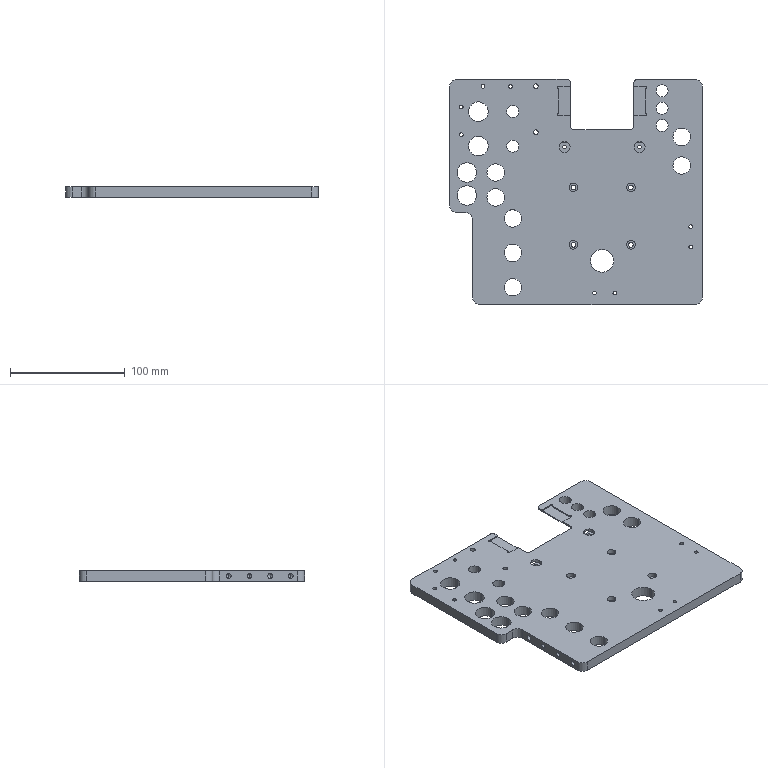NC program | NX | posted with a generic post | part box 220 x 196 x 9 mm
Lines 131 to 1017 of 7489:
(ZLEVEL_PROFILE , TOOL : D10)
N236 T15 M6
N238 G54
N240 G17 G0 G90 X56.431 Y-103.1 S9500 M3
N242 G43 Z30. H15
N244 Z1.5
N246 G94 G1 X10. Z-0.933 F1000.
N248 X-84. F3200.
N250 G2 X-95.1 Y-92. R11.1
N252 G1 Y-24.
N254 G3 X-96. Y-23.1 R0.9
N256 G1 X-104.
N258 G2 X-115.1 Y-12. R11.1
N260 G1 Y92.
N262 G2 X-104. Y103.1 R11.1
N264 G1 X-7.8
N266 G2 X0.3 Y95. R8.1
N268 G1 Y92.
N270 G2 X0.275 Y91.491 R5.1
N272 G1 Y66.909
N274 G2 X0.3 Y66.4 R5.1
N276 G1 Y59.5
N278 X45.15
N280 Y66.4
N282 G2 X45.175 Y66.909 R5.1
N284 G1 Y91.491
N286 G2 X45.15 Y92. R5.1
N288 G1 Y95.
N290 G2 X53.25 Y103.1 R8.1
N292 G1 X104.
N294 G2 X115.1 Y92. R11.1
N296 G1 Y-92.
N298 G2 X104. Y-103.1 R11.1
N300 G1 X10.
N302 X-43.471 Z-1.867
N304 X-84.
N306 G2 X-95.1 Y-92. R11.1
N308 G1 Y-24.
N310 G3 X-96. Y-23.1 R0.9
N312 G1 X-104.
N314 G2 X-115.1 Y-12. R11.1
N316 G1 Y92.
N318 G2 X-104. Y103.1 R11.1
N320 G1 X-7.8
N322 G2 X0.3 Y95. R8.1
N324 G1 Y59.5
N326 X45.15
N328 Y95.
N330 G2 X53.25 Y103.1 R8.1
N332 G1 X104.
N334 G2 X115.1 Y92. R11.1
N336 G1 Y-92.
N338 G2 X104. Y-103.1 R11.1
N340 G1 X10.
N342 X-43.471 Z-2.8
N344 X-84.
N346 G2 X-95.1 Y-92. R11.1
N348 G1 Y-24.
N350 G3 X-96. Y-23.1 R0.9
N352 G1 X-104.
N354 G2 X-115.1 Y-12. R11.1
N356 G1 Y92.
N358 G2 X-104. Y103.1 R11.1
N360 G1 X-7.8
N362 G2 X0.3 Y95. R8.1
N364 G1 Y59.5
N366 X45.15
N368 Y95.
N370 G2 X53.25 Y103.1 R8.1
N372 G1 X104.
N374 G2 X115.1 Y92. R11.1
N376 G1 Y-92.
N378 G2 X104. Y-103.1 R11.1
N380 G1 X10.
N382 X-43.471 Z-3.733
N384 X-84.
N386 G2 X-95.1 Y-92. R11.1
N388 G1 Y-24.
N390 G3 X-96. Y-23.1 R0.9
N392 G1 X-104.
N394 G2 X-115.1 Y-12. R11.1
N396 G1 Y92.
N398 G2 X-104. Y103.1 R11.1
N400 G1 X-7.8
N402 G2 X0.3 Y95. R8.1
N404 G1 Y59.5
N406 X45.15
N408 Y95.
N410 G2 X53.25 Y103.1 R8.1
N412 G1 X104.
N414 G2 X115.1 Y92. R11.1
N416 G1 Y-92.
N418 G2 X104. Y-103.1 R11.1
N420 G1 X10.
N422 X-43.471 Z-4.667
N424 X-84.
N426 G2 X-95.1 Y-92. R11.1
N428 G1 Y-24.
N430 G3 X-96. Y-23.1 R0.9
N432 G1 X-104.
N434 G2 X-115.1 Y-12. R11.1
N436 G1 Y92.
N438 G2 X-104. Y103.1 R11.1
N440 G1 X-7.8
N442 G2 X0.3 Y95. R8.1
N444 G1 Y59.5
N446 X45.15
N448 Y95.
N450 G2 X53.25 Y103.1 R8.1
N452 G1 X104.
N454 G2 X115.1 Y92. R11.1
N456 G1 Y-92.
N458 G2 X104. Y-103.1 R11.1
N460 G1 X10.
N462 X-43.471 Z-5.6
N464 X-84.
N466 G2 X-95.1 Y-92. R11.1
N468 G1 Y-24.
N470 G3 X-96. Y-23.1 R0.9
N472 G1 X-104.
N474 G2 X-115.1 Y-12. R11.1
N476 G1 Y92.
N478 G2 X-104. Y103.1 R11.1
N480 G1 X-7.8
N482 G2 X0.3 Y95. R8.1
N484 G1 Y59.5
N486 X45.15
N488 Y95.
N490 G2 X53.25 Y103.1 R8.1
N492 G1 X104.
N494 G2 X115.1 Y92. R11.1
N496 G1 Y-92.
N498 G2 X104. Y-103.1 R11.1
N500 G1 X10.
N502 X-43.471 Z-6.533
N504 X-84.
N506 G2 X-95.1 Y-92. R11.1
N508 G1 Y-24.
N510 G3 X-96. Y-23.1 R0.9
N512 G1 X-104.
N514 G2 X-115.1 Y-12. R11.1
N516 G1 Y92.
N518 G2 X-104. Y103.1 R11.1
N520 G1 X-7.8
N522 G2 X0.3 Y95. R8.1
N524 G1 Y59.5
N526 X45.15
N528 Y95.
N530 G2 X53.25 Y103.1 R8.1
N532 G1 X104.
N534 G2 X115.1 Y92. R11.1
N536 G1 Y-92.
N538 G2 X104. Y-103.1 R11.1
N540 G1 X10.
N542 X-43.471 Z-7.467
N544 X-84.
N546 G2 X-95.1 Y-92. R11.1
N548 G1 Y-24.
N550 G3 X-96. Y-23.1 R0.9
N552 G1 X-104.
N554 G2 X-115.1 Y-12. R11.1
N556 G1 Y92.
N558 G2 X-104. Y103.1 R11.1
N560 G1 X-7.8
N562 G2 X0.3 Y95. R8.1
N564 G1 Y59.5
N566 X45.15
N568 Y95.
N570 G2 X53.25 Y103.1 R8.1
N572 G1 X104.
N574 G2 X115.1 Y92. R11.1
N576 G1 Y-92.
N578 G2 X104. Y-103.1 R11.1
N580 G1 X10.
N582 X-43.471 Z-8.4
N584 X-84.
N586 G2 X-95.1 Y-92. R11.1
N588 G1 Y-24.
N590 G3 X-96. Y-23.1 R0.9
N592 G1 X-104.
N594 G2 X-115.1 Y-12. R11.1
N596 G1 Y92.
N598 G2 X-104. Y103.1 R11.1
N600 G1 X-7.8
N602 G2 X0.3 Y95. R8.1
N604 G1 Y59.5
N606 X45.15
N608 Y95.
N610 G2 X53.25 Y103.1 R8.1
N612 G1 X104.
N614 G2 X115.1 Y92. R11.1
N616 G1 Y-92.
N618 G2 X104. Y-103.1 R11.1
N620 G1 X-43.471
N622 Z-6.9
N624 G0 Z30.
(ZLEVEL_PROFILE_COPY , TOOL : D10)
N626 X-85.581 Y73.328
N628 Z1.5
N630 G1 X-86.277 Y73.183 Z1.463 F1000.
N632 X-87.297 Y72.547 Z1.4
N634 X-88.035 Y71.598 Z1.337
N636 X-88.4 Y70.453 Z1.274
N638 Y69.995 Z1.25
N640 X-88.399 Y69.543 Z1.226
N642 X-88.219 Y68.816 Z1.187
N644 X-87.797 Y68.015 Z1.139
N646 X-87.016 Y67.225 Z1.081
N648 X-86.024 Y66.727 Z1.023
N650 X-84.925 Y66.571 Z0.965
N652 X-83.833 Y66.774 Z0.907
N654 X-82.864 Y67.316 Z0.848
N656 X-82.236 Y67.968 Z0.801
N658 X-81.82 Y68.716 Z0.756
N660 X-81.601 Y69.543 Z0.711
N662 X-81.599 Y70.448 Z0.664
N664 X-81.861 Y71.383 Z0.613
N666 X-82.375 Y72.207 Z0.562
N668 X-83.098 Y72.855 Z0.511
N670 X-83.911 Y73.253 Z0.464
N672 X-85.101 Y73.429 Z0.401
N674 X-86.277 Y73.183 Z0.338
N676 X-87.297 Y72.547 Z0.275
N678 X-88.035 Y71.598 Z0.212
N680 X-88.4 Y70.453 Z0.149
N682 Y69.995 Z0.125
N684 X-88.399 Y69.543 Z0.101
N686 X-88.219 Y68.816 Z0.062
N688 X-87.797 Y68.015 Z0.014
N690 X-87.016 Y67.225 Z-0.044
N692 X-86.024 Y66.727 Z-0.102
N694 X-84.925 Y66.571 Z-0.16
N696 X-83.833 Y66.774 Z-0.218
N698 X-82.864 Y67.316 Z-0.277
N700 X-82.236 Y67.968 Z-0.324
N702 X-81.82 Y68.716 Z-0.369
N704 X-81.601 Y69.543 Z-0.414
N706 X-81.599 Y70.448 Z-0.461
N708 X-81.861 Y71.383 Z-0.512
N710 X-82.375 Y72.207 Z-0.563
N712 X-83.098 Y72.855 Z-0.614
N714 X-83.911 Y73.253 Z-0.661
N716 X-85.101 Y73.429 Z-0.724
N718 X-86.277 Y73.183 Z-0.787
N720 X-87.297 Y72.547 Z-0.85
N722 X-88.035 Y71.598 Z-0.913
N724 X-88.4 Y70.453 Z-0.976
N726 Y70. Z-1.
N728 Y69.995 F2000.
N730 G3 X-84.995 Y66.6 R3.4
N732 X-88.4 Y70. R-3.4
N734 G1 X-88.383 Y69.661 Z-1.021
N736 X-88.348 Y69.41 Z-1.037
N738 X-88.315 Y69.243 Z-1.048
N740 X-88.23 Y68.939 Z-1.067
N742 X-88.142 Y68.701 Z-1.083
N744 X-88.063 Y68.525 Z-1.095
N746 X-87.915 Y68.25 Z-1.115
N748 X-87.776 Y68.037 Z-1.131
N750 X-87.658 Y67.88 Z-1.143
N752 X-87.453 Y67.645 Z-1.162
N754 X-87.27 Y67.469 Z-1.178
N756 X-87.12 Y67.342 Z-1.19
N758 X-86.867 Y67.159 Z-1.21
N760 X-86.65 Y67.027 Z-1.226
N762 X-86.475 Y66.937 Z-1.238
N764 X-86.188 Y66.814 Z-1.258
N766 X-85.947 Y66.735 Z-1.273
N768 X-85.757 Y66.685 Z-1.286
N770 X-85.449 Y66.63 Z-1.305
N772 X-85.197 Y66.606 Z-1.321
N774 X-85. Y66.6 Z-1.333
N776 X-84.688 Y66.614 Z-1.353
N778 X-84.436 Y66.647 Z-1.369
N780 X-84.243 Y66.685 Z-1.381
N782 X-83.943 Y66.769 Z-1.4
N784 X-83.704 Y66.857 Z-1.416
N786 X-83.525 Y66.937 Z-1.429
N788 X-83.25 Y67.085 Z-1.448
N790 X-83.037 Y67.224 Z-1.464
N792 X-82.88 Y67.342 Z-1.476
N794 X-82.645 Y67.547 Z-1.496
N796 X-82.469 Y67.73 Z-1.512
N798 X-82.342 Y67.88 Z-1.524
N800 X-82.159 Y68.133 Z-1.543
N802 X-82.027 Y68.35 Z-1.559
N804 X-81.937 Y68.525 Z-1.571
N806 X-81.814 Y68.812 Z-1.591
N808 X-81.735 Y69.053 Z-1.607
N810 X-81.685 Y69.243 Z-1.619
N812 X-81.63 Y69.551 Z-1.638
N814 X-81.606 Y69.803 Z-1.654
N816 X-81.6 Y70. Z-1.667
N818 X-81.614 Y70.312 Z-1.686
N820 X-81.647 Y70.564 Z-1.702
N822 X-81.685 Y70.757 Z-1.714
N824 X-81.769 Y71.057 Z-1.734
N826 X-81.857 Y71.296 Z-1.75
N828 X-81.937 Y71.475 Z-1.762
N830 X-82.085 Y71.75 Z-1.781
N832 X-82.224 Y71.963 Z-1.797
N834 X-82.342 Y72.12 Z-1.81
N836 X-82.547 Y72.355 Z-1.829
N838 X-82.73 Y72.531 Z-1.845
N840 X-82.88 Y72.658 Z-1.857
N842 X-83.133 Y72.841 Z-1.877
N844 X-83.35 Y72.973 Z-1.892
N846 X-83.525 Y73.063 Z-1.905
N848 X-83.812 Y73.186 Z-1.924
N850 X-84.053 Y73.265 Z-1.94
N852 X-84.243 Y73.315 Z-1.952
N854 X-84.619 Y73.379 Z-1.976
N856 X-85. Y73.4 Z-2.
N858 G3 X-88.4 Y70. R3.4
N860 G1 X-88.383 Y69.661 Z-2.021
N862 X-88.348 Y69.41 Z-2.037
N864 X-88.315 Y69.243 Z-2.048
N866 X-88.23 Y68.939 Z-2.067
N868 X-88.142 Y68.701 Z-2.083
N870 X-88.063 Y68.525 Z-2.095
N872 X-87.915 Y68.25 Z-2.115
N874 X-87.776 Y68.037 Z-2.131
N876 X-87.658 Y67.88 Z-2.143
N878 X-87.453 Y67.645 Z-2.162
N880 X-87.27 Y67.469 Z-2.178
N882 X-87.12 Y67.342 Z-2.19
N884 X-86.867 Y67.159 Z-2.21
N886 X-86.65 Y67.027 Z-2.226
N888 X-86.475 Y66.937 Z-2.238
N890 X-86.188 Y66.814 Z-2.258
N892 X-85.947 Y66.735 Z-2.273
N894 X-85.757 Y66.685 Z-2.286
N896 X-85.449 Y66.63 Z-2.305
N898 X-85.197 Y66.606 Z-2.321
N900 X-85. Y66.6 Z-2.333
N902 X-84.688 Y66.614 Z-2.353
N904 X-84.436 Y66.647 Z-2.369
N906 X-84.243 Y66.685 Z-2.381
N908 X-83.943 Y66.769 Z-2.4
N910 X-83.704 Y66.857 Z-2.416
N912 X-83.525 Y66.937 Z-2.429
N914 X-83.25 Y67.085 Z-2.448
N916 X-83.037 Y67.224 Z-2.464
N918 X-82.88 Y67.342 Z-2.476
N920 X-82.645 Y67.547 Z-2.496
N922 X-82.469 Y67.73 Z-2.512
N924 X-82.342 Y67.88 Z-2.524
N926 X-82.159 Y68.133 Z-2.543
N928 X-82.027 Y68.35 Z-2.559
N930 X-81.937 Y68.525 Z-2.571
N932 X-81.814 Y68.812 Z-2.591
N934 X-81.735 Y69.053 Z-2.607
N936 X-81.685 Y69.243 Z-2.619
N938 X-81.63 Y69.551 Z-2.638
N940 X-81.606 Y69.803 Z-2.654
N942 X-81.6 Y70. Z-2.667
N944 X-81.614 Y70.312 Z-2.686
N946 X-81.647 Y70.564 Z-2.702
N948 X-81.685 Y70.757 Z-2.714
N950 X-81.769 Y71.057 Z-2.734
N952 X-81.857 Y71.296 Z-2.75
N954 X-81.937 Y71.475 Z-2.762
N956 X-82.085 Y71.75 Z-2.781
N958 X-82.224 Y71.963 Z-2.797
N960 X-82.342 Y72.12 Z-2.81
N962 X-82.547 Y72.355 Z-2.829
N964 X-82.73 Y72.531 Z-2.845
N966 X-82.88 Y72.658 Z-2.857
N968 X-83.133 Y72.841 Z-2.877
N970 X-83.35 Y72.973 Z-2.892
N972 X-83.525 Y73.063 Z-2.905
N974 X-83.812 Y73.186 Z-2.924
N976 X-84.053 Y73.265 Z-2.94
N978 X-84.243 Y73.315 Z-2.952
N980 X-84.619 Y73.379 Z-2.976
N982 X-85. Y73.4 Z-3.
N984 G3 X-88.4 Y70. R3.4
N986 G1 X-88.383 Y69.661 Z-3.021
N988 X-88.348 Y69.41 Z-3.037
N990 X-88.315 Y69.243 Z-3.048
N992 X-88.23 Y68.939 Z-3.067
N994 X-88.142 Y68.701 Z-3.083
N996 X-88.063 Y68.525 Z-3.095
N998 X-87.915 Y68.25 Z-3.115
N1000 X-87.776 Y68.037 Z-3.131
N1002 X-87.658 Y67.88 Z-3.143
N1004 X-87.453 Y67.645 Z-3.162
N1006 X-87.27 Y67.469 Z-3.178
N1008 X-87.12 Y67.342 Z-3.19
N1010 X-86.867 Y67.159 Z-3.21
N1012 X-86.65 Y67.027 Z-3.226
N1014 X-86.475 Y66.937 Z-3.238
N1016 X-86.188 Y66.814 Z-3.258
N1018 X-85.947 Y66.735 Z-3.273
N1020 X-85.757 Y66.685 Z-3.286
N1022 X-85.449 Y66.63 Z-3.305
N1024 X-85.197 Y66.606 Z-3.321
N1026 X-85. Y66.6 Z-3.333
N1028 X-84.688 Y66.614 Z-3.353
N1030 X-84.436 Y66.647 Z-3.369
N1032 X-84.243 Y66.685 Z-3.381
N1034 X-83.943 Y66.769 Z-3.4
N1036 X-83.704 Y66.857 Z-3.416
N1038 X-83.525 Y66.937 Z-3.429
N1040 X-83.25 Y67.085 Z-3.448
N1042 X-83.037 Y67.224 Z-3.464
N1044 X-82.88 Y67.342 Z-3.476
N1046 X-82.645 Y67.547 Z-3.496
N1048 X-82.469 Y67.73 Z-3.512
N1050 X-82.342 Y67.88 Z-3.524
N1052 X-82.159 Y68.133 Z-3.543
N1054 X-82.027 Y68.35 Z-3.559
N1056 X-81.937 Y68.525 Z-3.571
N1058 X-81.814 Y68.812 Z-3.591
N1060 X-81.735 Y69.053 Z-3.607
N1062 X-81.685 Y69.243 Z-3.619
N1064 X-81.63 Y69.551 Z-3.638
N1066 X-81.606 Y69.803 Z-3.654
N1068 X-81.6 Y70. Z-3.667
N1070 X-81.614 Y70.312 Z-3.686
N1072 X-81.647 Y70.564 Z-3.702
N1074 X-81.685 Y70.757 Z-3.714
N1076 X-81.769 Y71.057 Z-3.734
N1078 X-81.857 Y71.296 Z-3.75
N1080 X-81.937 Y71.475 Z-3.762
N1082 X-82.085 Y71.75 Z-3.781
N1084 X-82.224 Y71.963 Z-3.797
N1086 X-82.342 Y72.12 Z-3.81
N1088 X-82.547 Y72.355 Z-3.829
N1090 X-82.73 Y72.531 Z-3.845
N1092 X-82.88 Y72.658 Z-3.857
N1094 X-83.133 Y72.841 Z-3.877
N1096 X-83.35 Y72.973 Z-3.892
N1098 X-83.525 Y73.063 Z-3.905
N1100 X-83.812 Y73.186 Z-3.924
N1102 X-84.053 Y73.265 Z-3.94
N1104 X-84.243 Y73.315 Z-3.952
N1106 X-84.619 Y73.379 Z-3.976
N1108 X-85. Y73.4 Z-4.
N1110 G3 X-88.4 Y70. R3.4
N1112 G1 X-88.383 Y69.661 Z-4.021
N1114 X-88.348 Y69.41 Z-4.037
N1116 X-88.315 Y69.243 Z-4.048
N1118 X-88.23 Y68.939 Z-4.067
N1120 X-88.142 Y68.701 Z-4.083
N1122 X-88.063 Y68.525 Z-4.095
N1124 X-87.915 Y68.25 Z-4.115
N1126 X-87.776 Y68.037 Z-4.131
N1128 X-87.658 Y67.88 Z-4.143
N1130 X-87.453 Y67.645 Z-4.162
N1132 X-87.27 Y67.469 Z-4.178
N1134 X-87.12 Y67.342 Z-4.19
N1136 X-86.867 Y67.159 Z-4.21
N1138 X-86.65 Y67.027 Z-4.226
N1140 X-86.475 Y66.937 Z-4.238
N1142 X-86.188 Y66.814 Z-4.258
N1144 X-85.947 Y66.735 Z-4.273
N1146 X-85.757 Y66.685 Z-4.286
N1148 X-85.449 Y66.63 Z-4.305
N1150 X-85.197 Y66.606 Z-4.321
N1152 X-85. Y66.6 Z-4.333
N1154 X-84.688 Y66.614 Z-4.353
N1156 X-84.436 Y66.647 Z-4.369
N1158 X-84.243 Y66.685 Z-4.381
N1160 X-83.943 Y66.769 Z-4.4
N1162 X-83.704 Y66.857 Z-4.416
N1164 X-83.525 Y66.937 Z-4.429
N1166 X-83.25 Y67.085 Z-4.448
N1168 X-83.037 Y67.224 Z-4.464
N1170 X-82.88 Y67.342 Z-4.476
N1172 X-82.645 Y67.547 Z-4.496
N1174 X-82.469 Y67.73 Z-4.512
N1176 X-82.342 Y67.88 Z-4.524
N1178 X-82.159 Y68.133 Z-4.543
N1180 X-82.027 Y68.35 Z-4.559
N1182 X-81.937 Y68.525 Z-4.571
N1184 X-81.814 Y68.812 Z-4.591
N1186 X-81.735 Y69.053 Z-4.607
N1188 X-81.685 Y69.243 Z-4.619
N1190 X-81.63 Y69.551 Z-4.638
N1192 X-81.606 Y69.803 Z-4.654
N1194 X-81.6 Y70. Z-4.667
N1196 X-81.614 Y70.312 Z-4.686
N1198 X-81.647 Y70.564 Z-4.702
N1200 X-81.685 Y70.757 Z-4.714
N1202 X-81.769 Y71.057 Z-4.734
N1204 X-81.857 Y71.296 Z-4.75
N1206 X-81.937 Y71.475 Z-4.762
N1208 X-82.085 Y71.75 Z-4.781
N1210 X-82.224 Y71.963 Z-4.797
N1212 X-82.342 Y72.12 Z-4.81
N1214 X-82.547 Y72.355 Z-4.829
N1216 X-82.73 Y72.531 Z-4.845
N1218 X-82.88 Y72.658 Z-4.857
N1220 X-83.133 Y72.841 Z-4.877
N1222 X-83.35 Y72.973 Z-4.892
N1224 X-83.525 Y73.063 Z-4.905
N1226 X-83.812 Y73.186 Z-4.924
N1228 X-84.053 Y73.265 Z-4.94
N1230 X-84.243 Y73.315 Z-4.952
N1232 X-84.619 Y73.379 Z-4.976
N1234 X-85. Y73.4 Z-5.
N1236 G3 X-88.4 Y70. R3.4
N1238 G1 X-88.383 Y69.661 Z-5.021
N1240 X-88.348 Y69.41 Z-5.037
N1242 X-88.315 Y69.243 Z-5.048
N1244 X-88.23 Y68.939 Z-5.067
N1246 X-88.142 Y68.701 Z-5.083
N1248 X-88.063 Y68.525 Z-5.095
N1250 X-87.915 Y68.25 Z-5.115
N1252 X-87.776 Y68.037 Z-5.131
N1254 X-87.658 Y67.88 Z-5.143
N1256 X-87.453 Y67.645 Z-5.162
N1258 X-87.27 Y67.469 Z-5.178
N1260 X-87.12 Y67.342 Z-5.19
N1262 X-86.867 Y67.159 Z-5.21
N1264 X-86.65 Y67.027 Z-5.226
N1266 X-86.475 Y66.937 Z-5.238
N1268 X-86.188 Y66.814 Z-5.258
N1270 X-85.947 Y66.735 Z-5.273
N1272 X-85.757 Y66.685 Z-5.286
N1274 X-85.449 Y66.63 Z-5.305
N1276 X-85.197 Y66.606 Z-5.321
N1278 X-85. Y66.6 Z-5.333
N1280 X-84.688 Y66.614 Z-5.353
N1282 X-84.436 Y66.647 Z-5.369
N1284 X-84.243 Y66.685 Z-5.381
N1286 X-83.943 Y66.769 Z-5.4
N1288 X-83.704 Y66.857 Z-5.416
N1290 X-83.525 Y66.937 Z-5.429
N1292 X-83.25 Y67.085 Z-5.448
N1294 X-83.037 Y67.224 Z-5.464
N1296 X-82.88 Y67.342 Z-5.476
N1298 X-82.645 Y67.547 Z-5.496
N1300 X-82.469 Y67.73 Z-5.512
N1302 X-82.342 Y67.88 Z-5.524
N1304 X-82.159 Y68.133 Z-5.543
N1306 X-82.027 Y68.35 Z-5.559
N1308 X-81.937 Y68.525 Z-5.571
N1310 X-81.814 Y68.812 Z-5.591
N1312 X-81.735 Y69.053 Z-5.607
N1314 X-81.685 Y69.243 Z-5.619
N1316 X-81.63 Y69.551 Z-5.638
N1318 X-81.606 Y69.803 Z-5.654
N1320 X-81.6 Y70. Z-5.667
N1322 X-81.614 Y70.312 Z-5.686
N1324 X-81.647 Y70.564 Z-5.702
N1326 X-81.685 Y70.757 Z-5.714
N1328 X-81.769 Y71.057 Z-5.734
N1330 X-81.857 Y71.296 Z-5.75
N1332 X-81.937 Y71.475 Z-5.762
N1334 X-82.085 Y71.75 Z-5.781
N1336 X-82.224 Y71.963 Z-5.797
N1338 X-82.342 Y72.12 Z-5.81
N1340 X-82.547 Y72.355 Z-5.829
N1342 X-82.73 Y72.531 Z-5.845
N1344 X-82.88 Y72.658 Z-5.857
N1346 X-83.133 Y72.841 Z-5.877
N1348 X-83.35 Y72.973 Z-5.892
N1350 X-83.525 Y73.063 Z-5.905
N1352 X-83.812 Y73.186 Z-5.924
N1354 X-84.053 Y73.265 Z-5.94
N1356 X-84.243 Y73.315 Z-5.952
N1358 X-84.619 Y73.379 Z-5.976
N1360 X-85. Y73.4 Z-6.
N1362 G3 X-88.4 Y70. R3.4
N1364 G1 X-88.383 Y69.661 Z-6.021
N1366 X-88.348 Y69.41 Z-6.037
N1368 X-88.315 Y69.243 Z-6.048
N1370 X-88.23 Y68.939 Z-6.067
N1372 X-88.142 Y68.701 Z-6.083
N1374 X-88.063 Y68.525 Z-6.095
N1376 X-87.915 Y68.25 Z-6.115
N1378 X-87.776 Y68.037 Z-6.131
N1380 X-87.658 Y67.88 Z-6.143
N1382 X-87.453 Y67.645 Z-6.162
N1384 X-87.27 Y67.469 Z-6.178
N1386 X-87.12 Y67.342 Z-6.19
N1388 X-86.867 Y67.159 Z-6.21
N1390 X-86.65 Y67.027 Z-6.226
N1392 X-86.475 Y66.937 Z-6.238
N1394 X-86.188 Y66.814 Z-6.258
N1396 X-85.947 Y66.735 Z-6.273
N1398 X-85.757 Y66.685 Z-6.286
N1400 X-85.449 Y66.63 Z-6.305
N1402 X-85.197 Y66.606 Z-6.321
N1404 X-85. Y66.6 Z-6.333
N1406 X-84.688 Y66.614 Z-6.353
N1408 X-84.436 Y66.647 Z-6.369
N1410 X-84.243 Y66.685 Z-6.381
N1412 X-83.943 Y66.769 Z-6.4
N1414 X-83.704 Y66.857 Z-6.416
N1416 X-83.525 Y66.937 Z-6.429
N1418 X-83.25 Y67.085 Z-6.448
N1420 X-83.037 Y67.224 Z-6.464
N1422 X-82.88 Y67.342 Z-6.476
N1424 X-82.645 Y67.547 Z-6.496
N1426 X-82.469 Y67.73 Z-6.512
N1428 X-82.342 Y67.88 Z-6.524
N1430 X-82.159 Y68.133 Z-6.543
N1432 X-82.027 Y68.35 Z-6.559
N1434 X-81.937 Y68.525 Z-6.571
N1436 X-81.814 Y68.812 Z-6.591
N1438 X-81.735 Y69.053 Z-6.607
N1440 X-81.685 Y69.243 Z-6.619
N1442 X-81.63 Y69.551 Z-6.638
N1444 X-81.606 Y69.803 Z-6.654
N1446 X-81.6 Y70. Z-6.667
N1448 X-81.614 Y70.312 Z-6.686
N1450 X-81.647 Y70.564 Z-6.702
N1452 X-81.685 Y70.757 Z-6.714
N1454 X-81.769 Y71.057 Z-6.734
N1456 X-81.857 Y71.296 Z-6.75
N1458 X-81.937 Y71.475 Z-6.762
N1460 X-82.085 Y71.75 Z-6.781
N1462 X-82.224 Y71.963 Z-6.797
N1464 X-82.342 Y72.12 Z-6.81
N1466 X-82.547 Y72.355 Z-6.829
N1468 X-82.73 Y72.531 Z-6.845
N1470 X-82.88 Y72.658 Z-6.857
N1472 X-83.133 Y72.841 Z-6.877
N1474 X-83.35 Y72.973 Z-6.892
N1476 X-83.525 Y73.063 Z-6.905
N1478 X-83.812 Y73.186 Z-6.924
N1480 X-84.053 Y73.265 Z-6.94
N1482 X-84.243 Y73.315 Z-6.952
N1484 X-84.619 Y73.379 Z-6.976
N1486 X-85. Y73.4 Z-7.
N1488 G3 X-88.4 Y70. R3.4
N1490 G1 X-88.383 Y69.661 Z-7.021
N1492 X-88.348 Y69.41 Z-7.037
N1494 X-88.315 Y69.243 Z-7.048
N1496 X-88.23 Y68.939 Z-7.067
N1498 X-88.142 Y68.701 Z-7.083
N1500 X-88.063 Y68.525 Z-7.095
N1502 X-87.915 Y68.25 Z-7.115
N1504 X-87.776 Y68.037 Z-7.131
N1506 X-87.658 Y67.88 Z-7.143
N1508 X-87.453 Y67.645 Z-7.162
N1510 X-87.27 Y67.469 Z-7.178
N1512 X-87.12 Y67.342 Z-7.19
N1514 X-86.867 Y67.159 Z-7.21
N1516 X-86.65 Y67.027 Z-7.226
N1518 X-86.475 Y66.937 Z-7.238
N1520 X-86.188 Y66.814 Z-7.258
N1522 X-85.947 Y66.735 Z-7.273
N1524 X-85.757 Y66.685 Z-7.286
N1526 X-85.449 Y66.63 Z-7.305
N1528 X-85.197 Y66.606 Z-7.321
N1530 X-85. Y66.6 Z-7.333
N1532 X-84.688 Y66.614 Z-7.353
N1534 X-84.436 Y66.647 Z-7.369
N1536 X-84.243 Y66.685 Z-7.381
N1538 X-83.943 Y66.769 Z-7.4
N1540 X-83.704 Y66.857 Z-7.416
N1542 X-83.525 Y66.937 Z-7.429
N1544 X-83.25 Y67.085 Z-7.448
N1546 X-83.037 Y67.224 Z-7.464
N1548 X-82.88 Y67.342 Z-7.476
N1550 X-82.645 Y67.547 Z-7.496
N1552 X-82.469 Y67.73 Z-7.512
N1554 X-82.342 Y67.88 Z-7.524
N1556 X-82.159 Y68.133 Z-7.543
N1558 X-82.027 Y68.35 Z-7.559
N1560 X-81.937 Y68.525 Z-7.571
N1562 X-81.814 Y68.812 Z-7.591
N1564 X-81.735 Y69.053 Z-7.607
N1566 X-81.685 Y69.243 Z-7.619
N1568 X-81.63 Y69.551 Z-7.638
N1570 X-81.606 Y69.803 Z-7.654
N1572 X-81.6 Y70. Z-7.667
N1574 X-81.614 Y70.312 Z-7.686
N1576 X-81.647 Y70.564 Z-7.702
N1578 X-81.685 Y70.757 Z-7.714
N1580 X-81.769 Y71.057 Z-7.734
N1582 X-81.857 Y71.296 Z-7.75
N1584 X-81.937 Y71.475 Z-7.762
N1586 X-82.085 Y71.75 Z-7.781
N1588 X-82.224 Y71.963 Z-7.797
N1590 X-82.342 Y72.12 Z-7.81
N1592 X-82.547 Y72.355 Z-7.829
N1594 X-82.73 Y72.531 Z-7.845
N1596 X-82.88 Y72.658 Z-7.857
N1598 X-83.133 Y72.841 Z-7.877
N1600 X-83.35 Y72.973 Z-7.892
N1602 X-83.525 Y73.063 Z-7.905
N1604 X-83.812 Y73.186 Z-7.924
N1606 X-84.053 Y73.265 Z-7.94
N1608 X-84.243 Y73.315 Z-7.952
N1610 X-84.619 Y73.379 Z-7.976
N1612 X-85. Y73.4 Z-8.
N1614 G3 X-88.4 Y70. R3.4
N1616 G1 X-88.383 Y69.661 Z-8.021
N1618 X-88.348 Y69.41 Z-8.037
N1620 X-88.315 Y69.243 Z-8.048
N1622 X-88.23 Y68.939 Z-8.067
N1624 X-88.142 Y68.701 Z-8.083
N1626 X-88.063 Y68.525 Z-8.095
N1628 X-87.915 Y68.25 Z-8.115
N1630 X-87.776 Y68.037 Z-8.131
N1632 X-87.658 Y67.88 Z-8.143
N1634 X-87.453 Y67.645 Z-8.162
N1636 X-87.27 Y67.469 Z-8.178
N1638 X-87.12 Y67.342 Z-8.19
N1640 X-86.867 Y67.159 Z-8.21
N1642 X-86.65 Y67.027 Z-8.226
N1644 X-86.475 Y66.937 Z-8.238
N1646 X-86.188 Y66.814 Z-8.258
N1648 X-85.947 Y66.735 Z-8.273
N1650 X-85.757 Y66.685 Z-8.286
N1652 X-85.449 Y66.63 Z-8.305
N1654 X-85.197 Y66.606 Z-8.321
N1656 X-85. Y66.6 Z-8.333
N1658 X-84.688 Y66.614 Z-8.353
N1660 X-84.436 Y66.647 Z-8.369
N1662 X-84.243 Y66.685 Z-8.381
N1664 X-83.943 Y66.769 Z-8.4
N1666 X-83.704 Y66.857 Z-8.416
N1668 X-83.525 Y66.937 Z-8.429
N1670 X-83.25 Y67.085 Z-8.448
N1672 X-83.037 Y67.224 Z-8.464
N1674 X-82.88 Y67.342 Z-8.476
N1676 X-82.645 Y67.547 Z-8.496
N1678 X-82.469 Y67.73 Z-8.512
N1680 X-82.342 Y67.88 Z-8.524
N1682 X-82.159 Y68.133 Z-8.543
N1684 X-82.027 Y68.35 Z-8.559
N1686 X-81.937 Y68.525 Z-8.571
N1688 X-81.814 Y68.812 Z-8.591
N1690 X-81.735 Y69.053 Z-8.607
N1692 X-81.685 Y69.243 Z-8.619
N1694 X-81.63 Y69.551 Z-8.638
N1696 X-81.606 Y69.803 Z-8.654
N1698 X-81.6 Y70. Z-8.667
N1700 X-81.614 Y70.312 Z-8.686
N1702 X-81.647 Y70.564 Z-8.702
N1704 X-81.685 Y70.757 Z-8.714
N1706 X-81.769 Y71.057 Z-8.734
N1708 X-81.857 Y71.296 Z-8.75
N1710 X-81.937 Y71.475 Z-8.762
N1712 X-82.085 Y71.75 Z-8.781
N1714 X-82.224 Y71.963 Z-8.797
N1716 X-82.342 Y72.12 Z-8.81
N1718 X-82.547 Y72.355 Z-8.829
N1720 X-82.73 Y72.531 Z-8.845
N1722 X-82.88 Y72.658 Z-8.857
N1724 X-83.133 Y72.841 Z-8.877
N1726 X-83.35 Y72.973 Z-8.892
N1728 X-83.525 Y73.063 Z-8.905
N1730 X-83.812 Y73.186 Z-8.924
N1732 X-84.053 Y73.265 Z-8.94
N1734 X-84.243 Y73.315 Z-8.952
N1736 X-84.619 Y73.379 Z-8.976
N1738 X-85. Y73.4 Z-9.
N1740 G3 X-88.4 Y70. R3.4
N1742 X-85. Y73.4 R-3.4
N1744 G1 Z-7.5
N1746 G0 Z30.
N1748 X94.5 Y47.757
N1750 Z1.5
N1752 G1 Y48.001 Z1.487 F1000.
N1754 Y48.39 Z1.467
N1756 X94.256 Y49.144 Z1.425
N1758 X93.791 Y49.787 Z1.384
N1760 X93.15 Y50.254 Z1.342
N1762 X92.412 Y50.496 Z1.301
N1764 X91.42 Y50.463 Z1.249
N1766 X90.517 Y50.05 Z1.197
N1768 X89.842 Y49.321 Z1.145
N1770 X89.5 Y48.39 Z1.093
N1772 Y47.613 Z1.053
N1774 X89.632 Y47.108 Z1.025
N1776 X90.015 Y46.432 Z0.985
N1778 X90.683 Y45.84 Z0.938
N1780 X91.515 Y45.517 Z0.891
N1782 X92.408 Y45.503 Z0.844
N1784 X93.249 Y45.8 Z0.797
N1786 X93.858 Y46.283 Z0.757
N1788 X94.278 Y46.899 Z0.718
N1790 X94.5 Y47.612 Z0.679
N1792 Y48.001 Z0.658
N1794 Y48.39 Z0.638
N1796 X94.256 Y49.144 Z0.596
N1798 X93.791 Y49.787 Z0.555
N1800 X93.15 Y50.254 Z0.513
N1802 X92.412 Y50.496 Z0.472
N1804 X91.42 Y50.463 Z0.42
N1806 X90.517 Y50.05 Z0.368
N1808 X89.842 Y49.321 Z0.316
N1810 X89.5 Y48.39 Z0.264
N1812 Y47.613 Z0.224
N1814 X89.632 Y47.108 Z0.196
N1816 X90.015 Y46.432 Z0.155
N1818 X90.683 Y45.84 Z0.109
N1820 X91.515 Y45.517 Z0.062
N1822 X92.408 Y45.503 Z0.015
N1824 X93.249 Y45.8 Z-0.032
N1826 X93.858 Y46.283 Z-0.072
N1828 X94.278 Y46.899 Z-0.111
N1830 X94.5 Y47.612 Z-0.151
N1832 Y48.001 Z-0.171
N1834 Y48.39 Z-0.191
N1836 X94.256 Y49.144 Z-0.233
N1838 X93.791 Y49.787 Z-0.274
N1840 X93.15 Y50.254 Z-0.316
N1842 X92.412 Y50.496 Z-0.357
N1844 X91.42 Y50.463 Z-0.409
N1846 X90.517 Y50.05 Z-0.461
N1848 X89.842 Y49.321 Z-0.513
N1850 X89.5 Y48.39 Z-0.565
N1852 Y47.613 Z-0.606
N1854 X89.632 Y47.108 Z-0.633
N1856 X90.015 Y46.432 Z-0.674
N1858 X90.683 Y45.84 Z-0.72
N1860 X91.515 Y45.517 Z-0.767
N1862 X92.408 Y45.503 Z-0.814
N1864 X93.249 Y45.8 Z-0.861
N1866 X93.858 Y46.283 Z-0.901
N1868 X94.278 Y46.899 Z-0.941
N1870 X94.5 Y47.612 Z-0.98
N1872 Y48. Z-1.
N1874 Y48.001 F2000.
N1876 G3 X91.999 Y50.5 R2.5
N1878 X94.5 Y48. R-2.5
N1880 G1 X94.479 Y48.327 Z-1.028
N1882 X94.435 Y48.567 Z-1.049
N1884 X94.392 Y48.726 Z-1.063
N1886 X94.286 Y49.011 Z-1.088
N1888 X94.177 Y49.23 Z-1.109
N1890 X94.079 Y49.389 Z-1.125
N1892 X93.896 Y49.629 Z-1.151
N1894 X93.728 Y49.807 Z-1.171
N1896 X93.586 Y49.933 Z-1.188
N1898 X93.342 Y50.109 Z-1.213
N1900 X93.129 Y50.23 Z-1.234
N1902 X92.957 Y50.31 Z-1.25
N1904 X92.672 Y50.408 Z-1.275
N1906 X92.433 Y50.462 Z-1.296
N1908 X92.245 Y50.488 Z-1.313
N1910 X91.944 Y50.499 Z-1.338
N1912 X91.7 Y50.482 Z-1.359
N1914 X91.512 Y50.452 Z-1.375
N1916 X91.221 Y50.375 Z-1.4
N1918 X90.992 Y50.288 Z-1.421
N1920 X90.822 Y50.205 Z-1.438
N1922 X90.565 Y50.047 Z-1.463
N1924 X90.372 Y49.897 Z-1.484
N1926 X90.232 Y49.768 Z-1.5
N1928 X90.032 Y49.542 Z-1.525
N1930 X89.891 Y49.343 Z-1.546
N1932 X89.795 Y49.178 Z-1.563
N1934 X89.669 Y48.905 Z-1.588
N1936 X89.592 Y48.673 Z-1.609
N1938 X89.548 Y48.488 Z-1.625
N1940 X89.507 Y48.189 Z-1.65
N1942 X89.501 Y47.945 Z-1.671
N1944 X89.512 Y47.755 Z-1.688
N1946 X89.56 Y47.457 Z-1.713
N1948 X89.624 Y47.221 Z-1.734
N1950 X89.69 Y47.043 Z-1.75
N1952 X89.822 Y46.772 Z-1.775
N1954 X89.953 Y46.565 Z-1.796
N1956 X90.067 Y46.414 Z-1.813
N1958 X90.272 Y46.193 Z-1.838
N1960 X90.457 Y46.033 Z-1.859
N1962 X90.611 Y45.921 Z-1.875
N1964 X90.871 Y45.769 Z-1.9
N1966 X91.095 Y45.67 Z-1.921
N1968 X91.274 Y45.608 Z-1.938
N1970 X91.633 Y45.527 Z-1.969
N1972 X92. Y45.5 Z-2.
N1974 G3 X94.5 Y48. R2.5
N1976 G1 X94.479 Y48.327 Z-2.028
N1978 X94.435 Y48.567 Z-2.049
N1980 X94.392 Y48.726 Z-2.063
N1982 X94.286 Y49.011 Z-2.088
N1984 X94.177 Y49.23 Z-2.109
N1986 X94.079 Y49.389 Z-2.125
N1988 X93.896 Y49.629 Z-2.151
N1990 X93.728 Y49.807 Z-2.171
N1992 X93.586 Y49.933 Z-2.188
N1994 X93.342 Y50.109 Z-2.213
N1996 X93.129 Y50.23 Z-2.234